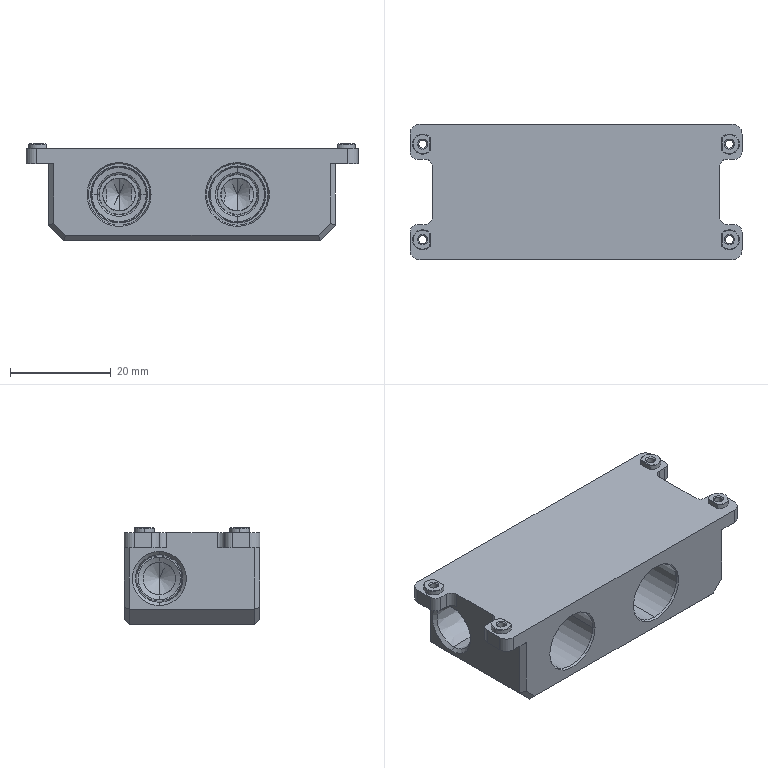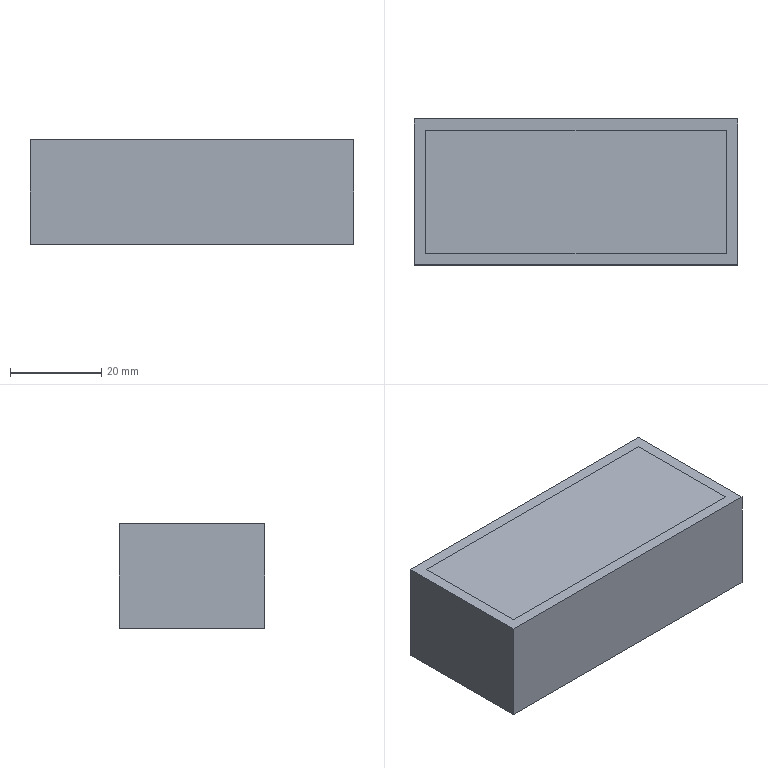CAM job | NX | 3+2 milling, drilling | part box 66 x 27 x 19.25 mm | stock box 71 x 32 x 23 mm
Tools:
number,name,description,diameter,corner_radius,flute_length,length,flutes
1,D50面刀,,80.0,0.0,50.0,75.0,2
2,D8开粗,,8.0,0.0,50.0,75.0,2
3,D8精光,,8.0,0.0,50.0,75.0,2
4,D3清角,,3.0,0.0,50.0,75.0,2
5,D3倒角刀,,3.0,0.0,35.0,50.0,2
12,D6,,6.0,0.0,50.0,75.0,2
6,D1.8钻头,,1.8,0.0,35.0,50.0,2
7,M2丝锥,,2.0,0.0,35.0,50.0,2
8,圆鼻刀,,4.0,0.5,50.0,75.0,2
9,D6.5钻头,,6.5,0.0,35.0,50.0,2
10,D8.4钻头,,8.4,0.0,35.0,50.0,2
11,NPT,,7.0,0.0,15.0,50.0,2
12,D12.5成型刀,,12.25,0.0,50.0,75.0,2
Operations:
program,operation,operation_type,tool,method,geometry_group,spindle_rpm,surface_speed,feed_per_tooth,feed_cut,feed_plunge,cut_length_mm,path_length_mm,cut_time_min,machine_time_min
G54,FLOOR_WALL,VolumeBased25DMillingOperation,D50面刀,METHOD,WORKPIECE,4500.0,706.0,0.0889,800.0,100.0,143.0,179.0,0.1787,0.1823
G54,ADAPTIVE_MILLING,CavityMilling,D8开粗,METHOD,WORKPIECE,7500.0,188.0,0.1667,2500.0,100.0,1898.863,3459.279,0.7499,0.906
G54,PLANAR_MILL,PlanarMilling,D8精光,METHOD,WORKPIECE,4500.0,113.0,0.0889,800.0,100.0,227.884,303.884,0.2849,0.2925
G54,PLANAR_MILL_1,PlanarMilling,D8精光,METHOD,WORKPIECE,4500.0,113.0,0.0889,800.0,100.0,114.223,291.993,0.1428,0.1606
G54,PLANAR_MILL_COPY,PlanarMilling,D3清角,METHOD,WORKPIECE,4500.0,42.0,0.0667,600.0,100.0,269.32,635.363,0.4489,0.4855
G54,PLANAR_MILL_COPY_COPY,PlanarMilling,D3清角,METHOD,WORKPIECE,4500.0,42.0,0.0444,400.0,100.0,202.248,544.538,0.5056,0.5398
G54,DRILLING,Operation,D3倒角刀,METHOD,WORKPIECE,3000.0,37.0,0.0333,200.0,0.0,16.0,211.044,0.08,0.0995
G54,PLANAR_MILL_2,PlanarMilling,D6,METHOD,WORKPIECE,3000.0,28.0,0.1,600.0,100.0,280.686,590.416,0.4678,0.4988
G54,DRILLING_COPY,Operation,D1.8钻头,METHOD,WORKPIECE,1600.0,9.0,0.025,80.0,0.0,30.0,239.044,0.375,0.3959
G54,DRILLING_COPY_COPY,Operation,M2丝锥,METHOD,WORKPIECE,300.0,1.0,0.2,120.0,0.0,28.0,235.044,0.2333,0.254
G54,ZLEVEL_PROFILE_STEEP,ZLevelMilling,圆鼻刀,METHOD,G54,6500.0,81.0,0.1538,2000.0,100.0,9083.938,9535.108,4.542,4.587
G55,DRILLING_1,Operation,D3倒角刀,METHOD,G55,2000.0,18.0,0.05,200.0,0.0,4.0,48.0,0.02,0.0244
G55,DRILLING_6,Operation,D6.5钻头,METHOD,G55,2000.0,40.0,0.05,200.0,0.0,49.0,138.0,0.245,0.2539
G55,DRILLING_2,Operation,D8.4钻头,METHOD,G55,1600.0,42.0,0.0625,200.0,0.0,15.0,70.0,0.075,0.0805
G55,PLANAR_MILL_4,PlanarMilling,D3倒角刀,METHOD,G55,4500.0,42.0,0.0667,600.0,100.0,34.127,72.127,0.0569,0.0607
G55,THREAD_MILLING,ThreadMilling,NPT,METHOD,G55,4500.0,84.0,0.0333,300.0,100.0,353.005,429.915,1.177,1.184
G56,FLOOR_WALL_1,VolumeBased25DMillingOperation,D50面刀,METHOD,G566,4500.0,706.0,0.1667,1500.0,100.0,948.0,1881.65,0.632,0.7254
G56,FLOOR_WALL_1_COPY,VolumeBased25DMillingOperation,D50面刀,METHOD,G566,4500.0,706.0,0.0667,600.0,100.0,158.0,192.0,0.2633,0.2667
G56,FLOOR_WALL_2,VolumeBased25DMillingOperation,D8开粗,METHOD,G566,6500.0,163.0,0.0769,1000.0,100.0,642.068,677.868,0.6421,0.6456
G56,FLOOR_WALL_2_COPY,VolumeBased25DMillingOperation,D8精光,METHOD,G566,6500.0,163.0,0.0462,600.0,100.0,658.807,694.807,1.098,1.102
G56,DRILLING_3,Operation,D3倒角刀,METHOD,G566,3000.0,28.0,0.0417,250.0,0.0,16.0,222.383,0.064,0.0846
G56,PLANAR_MILL_3_COPY,PlanarMilling,D3倒角刀,METHOD,G566,4500.0,42.0,0.0889,800.0,100.0,89.161,330.361,0.1115,0.1356
G56,PLANAR_MILL_3,PlanarMilling,D3倒角刀,METHOD,G566,4500.0,42.0,0.0889,800.0,100.0,213.239,253.639,0.2665,0.2706
G57,DRILLING_4,Operation,D3倒角刀,METHOD,WORKPIECE_1,3000.0,28.0,0.0417,250.0,0.0,8.0,82.691,0.032,0.0395
G57,DRILLING_4_COPY,Operation,D6.5钻头,METHOD,WORKPIECE_1,2000.0,40.0,0.05,200.0,0.0,55.5,177.691,0.2775,0.2897
G57,CAVITY_MILL,CavityMilling,D3清角,METHOD,WORKPIECE_1,1061.0,100.0,0.1178,250.0,100.0,2022.297,3994.924,8.089,8.287
G57,DRILLING_5,Operation,D12.5成型刀,METHOD,WORKPIECE_1,1800.0,69.0,0.0083,30.0,0.0,37.7,142.091,1.257,1.267